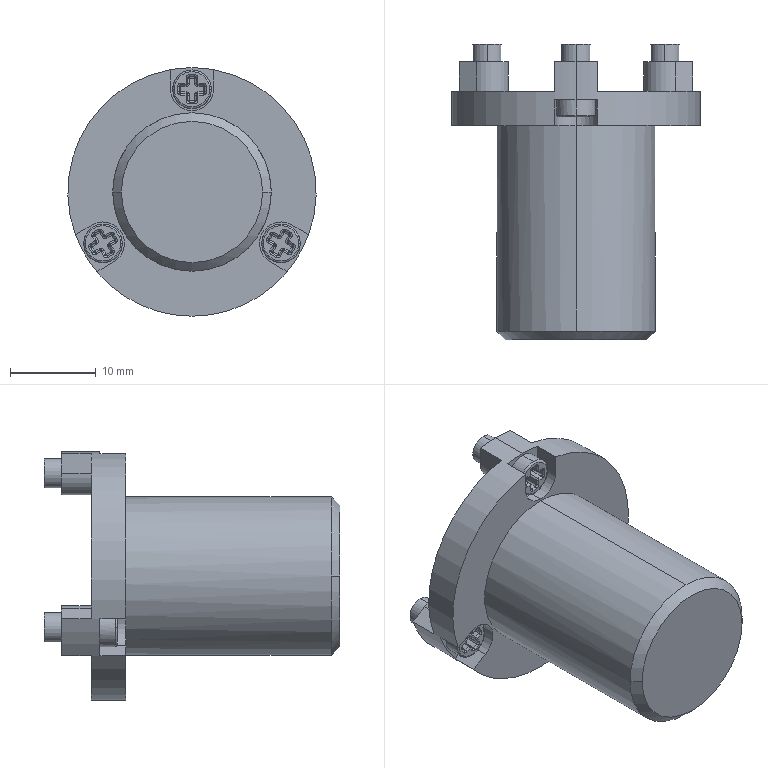Part | NX | 1 solid | 293 faces | box 29 x 34.5 x 29 mm | volume 8978 mm3 | cylinder 140 | plane 67 | torus 48 | sphere 36 | cone 2 | commonest cylinder face diameters 0.4 x114 5 x8 3.4 x6 4.5 x6 9 x2 18.5 x2